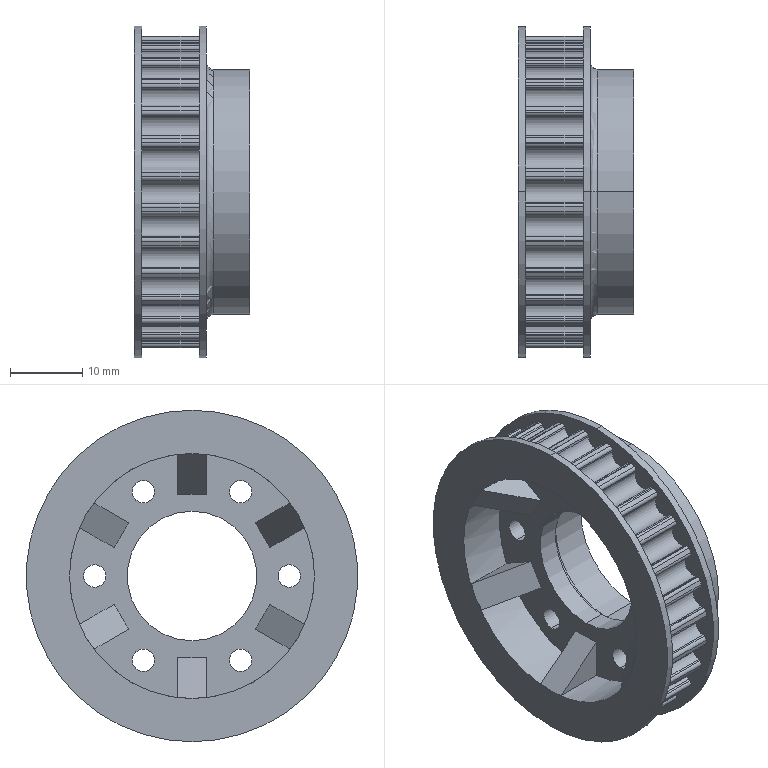Part | SolidWorks | features ICE 6, CirPattern 2, Cut 1, Fillet 1, RefAxis 1, Revolution 1 | 1 solid | 251 faces | box 16 x 46 x 46 mm | volume 10417 mm3 | cylinder 167 | plane 80 | torus 4 | commonest cylinder face diameters 0.96 x70 3.12 x41 43.416 x28 3.1 x12 34 x8 46 x4